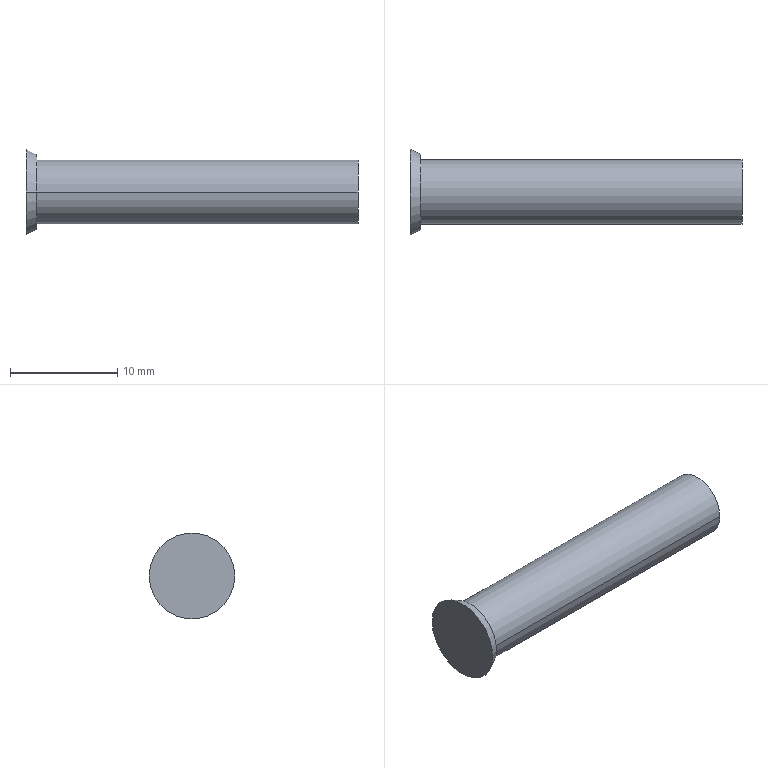Part | SolidWorks | features Revolution 1 | 1 solid | 7 faces | box 31 x 8 x 8 mm | volume 892.474 mm3 | plane 3 | cylinder 2 | cone 2 | commonest cylinder face diameters 6 x2
STEP:
#1=CARTESIAN_POINT('',(1.,3.,0.));
#2=VERTEX_POINT('',#1);
#3=CARTESIAN_POINT('',(1.,-3.,0.));
#4=VERTEX_POINT('',#3);
#5=CARTESIAN_POINT('',(1.,0.,0.));
#6=DIRECTION('',(1.,0.,0.));
#7=DIRECTION('',(0.,1.,0.));
#8=AXIS2_PLACEMENT_3D('',#5,#6,#7);
#9=CIRCLE('',#8,3.);
#10=EDGE_CURVE('',#2,#4,#9,.T.);
#11=ORIENTED_EDGE('',*,*,#10,.T.);
#12=CARTESIAN_POINT('',(31.,-3.,0.));
#13=VERTEX_POINT('',#12);
#14=CARTESIAN_POINT('',(31.,-3.,0.));
#15=DIRECTION('',(1.,0.,0.));
#16=VECTOR('',#15,1000.);
#17=LINE('',#14,#16);
#18=EDGE_CURVE('',#4,#13,#17,.T.);
#19=ORIENTED_EDGE('',*,*,#18,.T.);
#20=CARTESIAN_POINT('',(31.,3.,0.));
#21=VERTEX_POINT('',#20);
#22=CARTESIAN_POINT('',(31.,0.,0.));
#23=DIRECTION('',(1.,0.,0.));
#24=DIRECTION('',(0.,1.,0.));
#25=AXIS2_PLACEMENT_3D('',#22,#23,#24);
#26=CIRCLE('',#25,3.);
#27=EDGE_CURVE('',#21,#13,#26,.T.);
#28=ORIENTED_EDGE('',*,*,#27,.F.);
#29=CARTESIAN_POINT('',(31.,3.,0.));
#30=DIRECTION('',(1.,0.,0.));
#31=VECTOR('',#30,1000.);
#32=LINE('',#29,#31);
#33=EDGE_CURVE('',#2,#21,#32,.T.);
#34=ORIENTED_EDGE('',*,*,#33,.F.);
#35=EDGE_LOOP('',(#11,#19,#28,#34));
#36=FACE_OUTER_BOUND('',#35,.T.);
#37=CARTESIAN_POINT('',(31.,0.,0.));
#38=DIRECTION('',(1.,0.,0.));
#39=DIRECTION('',(0.,1.,0.));
#40=AXIS2_PLACEMENT_3D('',#37,#38,#39);
#41=CYLINDRICAL_SURFACE('',#40,3.);
#42=ADVANCED_FACE('',(#36),#41,.T.);
#43=CARTESIAN_POINT('',(1.,3.5,0.));
#44=VERTEX_POINT('',#43);
#45=CARTESIAN_POINT('',(1.,-3.5,0.));
#46=VERTEX_POINT('',#45);
#47=CARTESIAN_POINT('',(1.,0.,0.));
#48=DIRECTION('',(1.,0.,0.));
#49=DIRECTION('',(0.,1.,0.));
#50=AXIS2_PLACEMENT_3D('',#47,#48,#49);
#51=CIRCLE('',#50,3.5);
#52=EDGE_CURVE('',#44,#46,#51,.T.);
#53=ORIENTED_EDGE('',*,*,#52,.F.);
#54=CARTESIAN_POINT('',(0.,4.,0.));
#55=VERTEX_POINT('',#54);
#56=CARTESIAN_POINT('',(1.,3.5,0.));
#57=DIRECTION('',(-0.8944,0.4472,0.));
#58=VECTOR('',#57,1000.);
#59=LINE('',#56,#58);
#60=EDGE_CURVE('',#44,#55,#59,.T.);
#61=ORIENTED_EDGE('',*,*,#60,.T.);
#62=CARTESIAN_POINT('',(0.,-4.,0.));
#63=VERTEX_POINT('',#62);
#64=CARTESIAN_POINT('',(0.,0.,0.));
#65=DIRECTION('',(1.,0.,0.));
#66=DIRECTION('',(0.,1.,0.));
#67=AXIS2_PLACEMENT_3D('',#64,#65,#66);
#68=CIRCLE('',#67,4.);
#69=EDGE_CURVE('',#55,#63,#68,.T.);
#70=ORIENTED_EDGE('',*,*,#69,.T.);
#71=CARTESIAN_POINT('',(1.,-3.5,0.));
#72=DIRECTION('',(-0.8944,-0.4472,0.));
#73=VECTOR('',#72,1000.);
#74=LINE('',#71,#73);
#75=EDGE_CURVE('',#46,#63,#74,.T.);
#76=ORIENTED_EDGE('',*,*,#75,.F.);
#77=EDGE_LOOP('',(#53,#61,#70,#76));
#78=FACE_OUTER_BOUND('',#77,.T.);
#79=CARTESIAN_POINT('',(1.,0.,0.));
#80=DIRECTION('',(-1.,0.,0.));
#81=DIRECTION('',(0.,-1.,0.));
#82=AXIS2_PLACEMENT_3D('',#79,#80,#81);
#83=CONICAL_SURFACE('',#82,3.5,0.4636);
#84=ADVANCED_FACE('',(#78),#83,.T.);
#85=CARTESIAN_POINT('',(0.,0.,0.));
#86=DIRECTION('',(1.,0.,0.));
#87=DIRECTION('',(0.,1.,0.));
#88=AXIS2_PLACEMENT_3D('',#85,#86,#87);
#89=CIRCLE('',#88,4.);
#90=EDGE_CURVE('',#63,#55,#89,.T.);
#91=ORIENTED_EDGE('',*,*,#90,.F.);
#92=ORIENTED_EDGE('',*,*,#69,.F.);
#93=EDGE_LOOP('',(#91,#92));
#94=FACE_OUTER_BOUND('',#93,.T.);
#95=CARTESIAN_POINT('',(0.,0.,0.));
#96=DIRECTION('',(-1.,0.,0.));
#97=DIRECTION('',(0.,-1.,0.));
#98=AXIS2_PLACEMENT_3D('',#95,#96,#97);
#99=PLANE('',#98);
#100=ADVANCED_FACE('',(#94),#99,.T.);
#101=ORIENTED_EDGE('',*,*,#60,.F.);
#102=CARTESIAN_POINT('',(1.,0.,0.));
#103=DIRECTION('',(1.,0.,0.));
#104=DIRECTION('',(0.,1.,0.));
#105=AXIS2_PLACEMENT_3D('',#102,#103,#104);
#106=CIRCLE('',#105,3.5);
#107=EDGE_CURVE('',#46,#44,#106,.T.);
#108=ORIENTED_EDGE('',*,*,#107,.F.);
#109=ORIENTED_EDGE('',*,*,#75,.T.);
#110=ORIENTED_EDGE('',*,*,#90,.T.);
#111=EDGE_LOOP('',(#101,#108,#109,#110));
#112=FACE_OUTER_BOUND('',#111,.T.);
#113=CARTESIAN_POINT('',(1.,0.,0.));
#114=DIRECTION('',(-1.,0.,0.));
#115=DIRECTION('',(0.,-1.,0.));
#116=AXIS2_PLACEMENT_3D('',#113,#114,#115);
#117=CONICAL_SURFACE('',#116,3.5,0.4636);
#118=ADVANCED_FACE('',(#112),#117,.T.);
#119=ORIENTED_EDGE('',*,*,#107,.T.);
#120=ORIENTED_EDGE('',*,*,#52,.T.);
#121=EDGE_LOOP('',(#119,#120));
#122=FACE_OUTER_BOUND('',#121,.T.);
#123=ORIENTED_EDGE('',*,*,#10,.F.);
#124=CARTESIAN_POINT('',(1.,0.,0.));
#125=DIRECTION('',(1.,0.,0.));
#126=DIRECTION('',(0.,1.,0.));
#127=AXIS2_PLACEMENT_3D('',#124,#125,#126);
#128=CIRCLE('',#127,3.);
#129=EDGE_CURVE('',#4,#2,#128,.T.);
#130=ORIENTED_EDGE('',*,*,#129,.F.);
#131=EDGE_LOOP('',(#123,#130));
#132=FACE_BOUND('',#131,.T.);
#133=CARTESIAN_POINT('',(1.,3.5,0.));
#134=DIRECTION('',(1.,0.,0.));
#135=DIRECTION('',(0.,1.,0.));
#136=AXIS2_PLACEMENT_3D('',#133,#134,#135);
#137=PLANE('',#136);
#138=ADVANCED_FACE('',(#122,#132),#137,.T.);
#139=ORIENTED_EDGE('',*,*,#18,.F.);
#140=ORIENTED_EDGE('',*,*,#129,.T.);
#141=ORIENTED_EDGE('',*,*,#33,.T.);
#142=CARTESIAN_POINT('',(31.,0.,0.));
#143=DIRECTION('',(1.,0.,0.));
#144=DIRECTION('',(0.,1.,0.));
#145=AXIS2_PLACEMENT_3D('',#142,#143,#144);
#146=CIRCLE('',#145,3.);
#147=EDGE_CURVE('',#13,#21,#146,.T.);
#148=ORIENTED_EDGE('',*,*,#147,.F.);
#149=EDGE_LOOP('',(#139,#140,#141,#148));
#150=FACE_OUTER_BOUND('',#149,.T.);
#151=CARTESIAN_POINT('',(31.,0.,0.));
#152=DIRECTION('',(1.,0.,0.));
#153=DIRECTION('',(0.,1.,0.));
#154=AXIS2_PLACEMENT_3D('',#151,#152,#153);
#155=CYLINDRICAL_SURFACE('',#154,3.);
#156=ADVANCED_FACE('',(#150),#155,.T.);
#157=ORIENTED_EDGE('',*,*,#27,.T.);
#158=ORIENTED_EDGE('',*,*,#147,.T.);
#159=EDGE_LOOP('',(#157,#158));
#160=FACE_OUTER_BOUND('',#159,.T.);
#161=CARTESIAN_POINT('',(31.,3.,0.));
#162=DIRECTION('',(1.,0.,0.));
#163=DIRECTION('',(0.,1.,0.));
#164=AXIS2_PLACEMENT_3D('',#161,#162,#163);
#165=PLANE('',#164);
#166=ADVANCED_FACE('',(#160),#165,.T.);
#167=CLOSED_SHELL('',(#42,#84,#100,#118,#138,#156,#166));
#168=MANIFOLD_SOLID_BREP('',#167);
#169=CARTESIAN_POINT('',(0.,0.,0.));
#170=DIRECTION('',(0.,0.,1.));
#171=DIRECTION('',(1.,0.,0.));
#172=AXIS2_PLACEMENT_3D('',#169,#170,#171);
#173=(LENGTH_UNIT()NAMED_UNIT(*)SI_UNIT(.MILLI.,.METRE.));
#174=UNCERTAINTY_MEASURE_WITH_UNIT(LENGTH_MEASURE(0.00001),#173,'','');
#175=(NAMED_UNIT(*)PLANE_ANGLE_UNIT()SI_UNIT($,.RADIAN.));
#176=(NAMED_UNIT(*)SI_UNIT($,.STERADIAN.)SOLID_ANGLE_UNIT());
#177=(GEOMETRIC_REPRESENTATION_CONTEXT(3)GLOBAL_UNCERTAINTY_ASSIGNED_CONTEXT((#174))GLOBAL_UNIT_ASSIGNED_CONTEXT((#173,#175,#176))REPRESENTATION_CONTEXT('',''));
#178=ADVANCED_BREP_SHAPE_REPRESENTATION('',(#168,#172),#177);